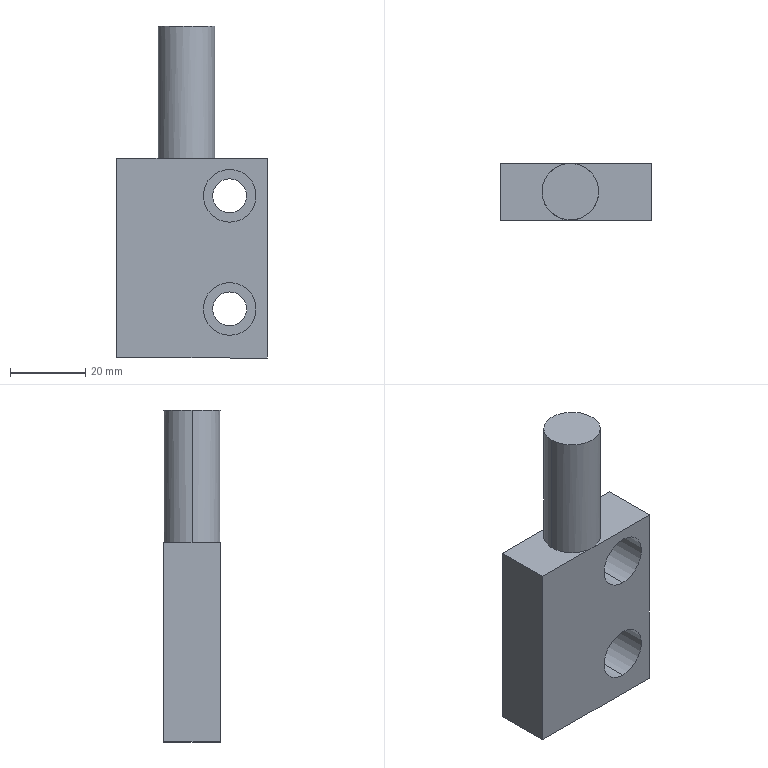Part | SolidWorks | features BaseBody 1 | 1 solid | 20 faces | box 40 x 15 x 88 mm | volume 34270 mm3 | cylinder 10 | plane 10 | commonest cylinder face diameters 9 x4 14 x4 15 x2
STEP:
#1=CARTESIAN_POINT('',(-340.,-80.,212.621));
#2=VERTEX_POINT('',#1);
#3=CARTESIAN_POINT('',(-340.,-80.,221.621));
#4=VERTEX_POINT('',#3);
#5=CARTESIAN_POINT('',(-340.,-80.,217.121));
#6=DIRECTION('',(0.,1.,0.));
#7=DIRECTION('',(0.,0.,-1.));
#8=AXIS2_PLACEMENT_3D('',#5,#6,#7);
#9=CIRCLE('',#8,4.5);
#10=EDGE_CURVE('',#2,#4,#9,.T.);
#11=ORIENTED_EDGE('',*,*,#10,.T.);
#12=CARTESIAN_POINT('',(-340.,-85.,221.621));
#13=VERTEX_POINT('',#12);
#14=CARTESIAN_POINT('',(-340.,-95.,221.621));
#15=DIRECTION('',(0.,-1.,0.));
#16=VECTOR('',#15,1000.);
#17=LINE('',#14,#16);
#18=EDGE_CURVE('',#4,#13,#17,.T.);
#19=ORIENTED_EDGE('',*,*,#18,.T.);
#20=CARTESIAN_POINT('',(-340.,-85.,212.621));
#21=VERTEX_POINT('',#20);
#22=CARTESIAN_POINT('',(-340.,-85.,217.121));
#23=DIRECTION('',(0.,1.,0.));
#24=DIRECTION('',(0.,0.,-1.));
#25=AXIS2_PLACEMENT_3D('',#22,#23,#24);
#26=CIRCLE('',#25,4.5);
#27=EDGE_CURVE('',#21,#13,#26,.T.);
#28=ORIENTED_EDGE('',*,*,#27,.F.);
#29=CARTESIAN_POINT('',(-340.,-95.,212.621));
#30=DIRECTION('',(0.,-1.,0.));
#31=VECTOR('',#30,1000.);
#32=LINE('',#29,#31);
#33=EDGE_CURVE('',#2,#21,#32,.T.);
#34=ORIENTED_EDGE('',*,*,#33,.F.);
#35=EDGE_LOOP('',(#11,#19,#28,#34));
#36=FACE_OUTER_BOUND('',#35,.T.);
#37=CARTESIAN_POINT('',(-340.,-95.,217.121));
#38=DIRECTION('',(0.,-1.,0.));
#39=DIRECTION('',(0.,0.,-1.));
#40=AXIS2_PLACEMENT_3D('',#37,#38,#39);
#41=CYLINDRICAL_SURFACE('',#40,4.5);
#42=ADVANCED_FACE('',(#36),#41,.F.);
#43=CARTESIAN_POINT('',(-340.,-80.,242.621));
#44=VERTEX_POINT('',#43);
#45=CARTESIAN_POINT('',(-340.,-80.,251.621));
#46=VERTEX_POINT('',#45);
#47=CARTESIAN_POINT('',(-340.,-80.,247.121));
#48=DIRECTION('',(0.,1.,0.));
#49=DIRECTION('',(0.,0.,-1.));
#50=AXIS2_PLACEMENT_3D('',#47,#48,#49);
#51=CIRCLE('',#50,4.5);
#52=EDGE_CURVE('',#44,#46,#51,.T.);
#53=ORIENTED_EDGE('',*,*,#52,.T.);
#54=CARTESIAN_POINT('',(-340.,-85.,251.621));
#55=VERTEX_POINT('',#54);
#56=CARTESIAN_POINT('',(-340.,-95.,251.621));
#57=DIRECTION('',(0.,-1.,0.));
#58=VECTOR('',#57,1000.);
#59=LINE('',#56,#58);
#60=EDGE_CURVE('',#46,#55,#59,.T.);
#61=ORIENTED_EDGE('',*,*,#60,.T.);
#62=CARTESIAN_POINT('',(-340.,-85.,242.621));
#63=VERTEX_POINT('',#62);
#64=CARTESIAN_POINT('',(-340.,-85.,247.121));
#65=DIRECTION('',(0.,1.,0.));
#66=DIRECTION('',(0.,0.,-1.));
#67=AXIS2_PLACEMENT_3D('',#64,#65,#66);
#68=CIRCLE('',#67,4.5);
#69=EDGE_CURVE('',#63,#55,#68,.T.);
#70=ORIENTED_EDGE('',*,*,#69,.F.);
#71=CARTESIAN_POINT('',(-340.,-95.,242.621));
#72=DIRECTION('',(0.,-1.,0.));
#73=VECTOR('',#72,1000.);
#74=LINE('',#71,#73);
#75=EDGE_CURVE('',#44,#63,#74,.T.);
#76=ORIENTED_EDGE('',*,*,#75,.F.);
#77=EDGE_LOOP('',(#53,#61,#70,#76));
#78=FACE_OUTER_BOUND('',#77,.T.);
#79=CARTESIAN_POINT('',(-340.,-95.,247.121));
#80=DIRECTION('',(0.,-1.,0.));
#81=DIRECTION('',(0.,0.,-1.));
#82=AXIS2_PLACEMENT_3D('',#79,#80,#81);
#83=CYLINDRICAL_SURFACE('',#82,4.5);
#84=ADVANCED_FACE('',(#78),#83,.F.);
#85=CARTESIAN_POINT('',(-359.,-87.5,292.121));
#86=VERTEX_POINT('',#85);
#87=CARTESIAN_POINT('',(-344.,-87.5,292.121));
#88=VERTEX_POINT('',#87);
#89=CARTESIAN_POINT('',(-351.5,-87.5,292.121));
#90=DIRECTION('',(0.,0.,-1.));
#91=DIRECTION('',(-1.,0.,0.));
#92=AXIS2_PLACEMENT_3D('',#89,#90,#91);
#93=CIRCLE('',#92,7.5);
#94=EDGE_CURVE('',#86,#88,#93,.T.);
#95=ORIENTED_EDGE('',*,*,#94,.T.);
#96=CARTESIAN_POINT('',(-344.,-87.5,257.121));
#97=VERTEX_POINT('',#96);
#98=CARTESIAN_POINT('',(-344.,-87.5,292.121));
#99=DIRECTION('',(0.,0.,-1.));
#100=VECTOR('',#99,1000.);
#101=LINE('',#98,#100);
#102=EDGE_CURVE('',#88,#97,#101,.T.);
#103=ORIENTED_EDGE('',*,*,#102,.T.);
#104=CARTESIAN_POINT('',(-351.5,-80.,257.121));
#105=VERTEX_POINT('',#104);
#106=CARTESIAN_POINT('',(-351.5,-87.5,257.121));
#107=DIRECTION('',(0.,0.,1.));
#108=DIRECTION('',(-1.,0.,0.));
#109=AXIS2_PLACEMENT_3D('',#106,#107,#108);
#110=CIRCLE('',#109,7.5);
#111=EDGE_CURVE('',#97,#105,#110,.T.);
#112=ORIENTED_EDGE('',*,*,#111,.T.);
#113=CARTESIAN_POINT('',(-359.,-87.5,257.121));
#114=VERTEX_POINT('',#113);
#115=CARTESIAN_POINT('',(-351.5,-87.5,257.121));
#116=DIRECTION('',(0.,0.,1.));
#117=DIRECTION('',(-1.,0.,0.));
#118=AXIS2_PLACEMENT_3D('',#115,#116,#117);
#119=CIRCLE('',#118,7.5);
#120=EDGE_CURVE('',#105,#114,#119,.T.);
#121=ORIENTED_EDGE('',*,*,#120,.T.);
#122=CARTESIAN_POINT('',(-359.,-87.5,292.121));
#123=DIRECTION('',(0.,0.,-1.));
#124=VECTOR('',#123,1000.);
#125=LINE('',#122,#124);
#126=EDGE_CURVE('',#86,#114,#125,.T.);
#127=ORIENTED_EDGE('',*,*,#126,.F.);
#128=EDGE_LOOP('',(#95,#103,#112,#121,#127));
#129=FACE_OUTER_BOUND('',#128,.T.);
#130=CARTESIAN_POINT('',(-351.5,-87.5,292.121));
#131=DIRECTION('',(0.,0.,-1.));
#132=DIRECTION('',(-1.,0.,0.));
#133=AXIS2_PLACEMENT_3D('',#130,#131,#132);
#134=CYLINDRICAL_SURFACE('',#133,7.5);
#135=ADVANCED_FACE('',(#129),#134,.T.);
#136=CARTESIAN_POINT('',(-340.,-85.,224.121));
#137=VERTEX_POINT('',#136);
#138=CARTESIAN_POINT('',(-340.,-85.,210.121));
#139=VERTEX_POINT('',#138);
#140=CARTESIAN_POINT('',(-340.,-85.,217.121));
#141=DIRECTION('',(0.,-1.,0.));
#142=DIRECTION('',(0.,0.,-1.));
#143=AXIS2_PLACEMENT_3D('',#140,#141,#142);
#144=CIRCLE('',#143,7.);
#145=EDGE_CURVE('',#137,#139,#144,.T.);
#146=ORIENTED_EDGE('',*,*,#145,.F.);
#147=CARTESIAN_POINT('',(-340.,-95.,224.121));
#148=VERTEX_POINT('',#147);
#149=CARTESIAN_POINT('',(-340.,-85.,224.121));
#150=DIRECTION('',(0.,-1.,0.));
#151=VECTOR('',#150,1000.);
#152=LINE('',#149,#151);
#153=EDGE_CURVE('',#137,#148,#152,.T.);
#154=ORIENTED_EDGE('',*,*,#153,.T.);
#155=CARTESIAN_POINT('',(-340.,-95.,210.121));
#156=VERTEX_POINT('',#155);
#157=CARTESIAN_POINT('',(-340.,-95.,217.121));
#158=DIRECTION('',(0.,-1.,0.));
#159=DIRECTION('',(0.,0.,-1.));
#160=AXIS2_PLACEMENT_3D('',#157,#158,#159);
#161=CIRCLE('',#160,7.);
#162=EDGE_CURVE('',#148,#156,#161,.T.);
#163=ORIENTED_EDGE('',*,*,#162,.T.);
#164=CARTESIAN_POINT('',(-340.,-85.,210.121));
#165=DIRECTION('',(0.,-1.,0.));
#166=VECTOR('',#165,1000.);
#167=LINE('',#164,#166);
#168=EDGE_CURVE('',#139,#156,#167,.T.);
#169=ORIENTED_EDGE('',*,*,#168,.F.);
#170=EDGE_LOOP('',(#146,#154,#163,#169));
#171=FACE_OUTER_BOUND('',#170,.T.);
#172=CARTESIAN_POINT('',(-340.,-85.,217.121));
#173=DIRECTION('',(0.,-1.,0.));
#174=DIRECTION('',(0.,0.,-1.));
#175=AXIS2_PLACEMENT_3D('',#172,#173,#174);
#176=CYLINDRICAL_SURFACE('',#175,7.);
#177=ADVANCED_FACE('',(#171),#176,.F.);
#178=CARTESIAN_POINT('',(-340.,-85.,254.121));
#179=VERTEX_POINT('',#178);
#180=CARTESIAN_POINT('',(-340.,-85.,240.121));
#181=VERTEX_POINT('',#180);
#182=CARTESIAN_POINT('',(-340.,-85.,247.121));
#183=DIRECTION('',(0.,-1.,0.));
#184=DIRECTION('',(0.,0.,-1.));
#185=AXIS2_PLACEMENT_3D('',#182,#183,#184);
#186=CIRCLE('',#185,7.);
#187=EDGE_CURVE('',#179,#181,#186,.T.);
#188=ORIENTED_EDGE('',*,*,#187,.F.);
#189=CARTESIAN_POINT('',(-340.,-95.,254.121));
#190=VERTEX_POINT('',#189);
#191=CARTESIAN_POINT('',(-340.,-85.,254.121));
#192=DIRECTION('',(0.,-1.,0.));
#193=VECTOR('',#192,1000.);
#194=LINE('',#191,#193);
#195=EDGE_CURVE('',#179,#190,#194,.T.);
#196=ORIENTED_EDGE('',*,*,#195,.T.);
#197=CARTESIAN_POINT('',(-340.,-95.,240.121));
#198=VERTEX_POINT('',#197);
#199=CARTESIAN_POINT('',(-340.,-95.,247.121));
#200=DIRECTION('',(0.,-1.,0.));
#201=DIRECTION('',(0.,0.,-1.));
#202=AXIS2_PLACEMENT_3D('',#199,#200,#201);
#203=CIRCLE('',#202,7.);
#204=EDGE_CURVE('',#190,#198,#203,.T.);
#205=ORIENTED_EDGE('',*,*,#204,.T.);
#206=CARTESIAN_POINT('',(-340.,-85.,240.121));
#207=DIRECTION('',(0.,-1.,0.));
#208=VECTOR('',#207,1000.);
#209=LINE('',#206,#208);
#210=EDGE_CURVE('',#181,#198,#209,.T.);
#211=ORIENTED_EDGE('',*,*,#210,.F.);
#212=EDGE_LOOP('',(#188,#196,#205,#211));
#213=FACE_OUTER_BOUND('',#212,.T.);
#214=CARTESIAN_POINT('',(-340.,-85.,247.121));
#215=DIRECTION('',(0.,-1.,0.));
#216=DIRECTION('',(0.,0.,-1.));
#217=AXIS2_PLACEMENT_3D('',#214,#215,#216);
#218=CYLINDRICAL_SURFACE('',#217,7.);
#219=ADVANCED_FACE('',(#213),#218,.F.);
#220=CARTESIAN_POINT('',(-370.,-80.,257.121));
#221=VERTEX_POINT('',#220);
#222=CARTESIAN_POINT('',(-370.,-80.,204.121));
#223=VERTEX_POINT('',#222);
#224=CARTESIAN_POINT('',(-370.,-80.,204.121));
#225=DIRECTION('',(0.,0.,-1.));
#226=VECTOR('',#225,1000.);
#227=LINE('',#224,#226);
#228=EDGE_CURVE('',#221,#223,#227,.T.);
#229=ORIENTED_EDGE('',*,*,#228,.F.);
#230=CARTESIAN_POINT('',(-330.,-80.,257.121));
#231=DIRECTION('',(-1.,0.,0.));
#232=VECTOR('',#231,1000.);
#233=LINE('',#230,#232);
#234=EDGE_CURVE('',#105,#221,#233,.T.);
#235=ORIENTED_EDGE('',*,*,#234,.F.);
#236=CARTESIAN_POINT('',(-330.,-80.,257.121));
#237=VERTEX_POINT('',#236);
#238=CARTESIAN_POINT('',(-330.,-80.,257.121));
#239=DIRECTION('',(-1.,0.,0.));
#240=VECTOR('',#239,1000.);
#241=LINE('',#238,#240);
#242=EDGE_CURVE('',#237,#105,#241,.T.);
#243=ORIENTED_EDGE('',*,*,#242,.F.);
#244=CARTESIAN_POINT('',(-330.,-80.,204.121));
#245=VERTEX_POINT('',#244);
#246=CARTESIAN_POINT('',(-330.,-80.,204.121));
#247=DIRECTION('',(0.,0.,1.));
#248=VECTOR('',#247,1000.);
#249=LINE('',#246,#248);
#250=EDGE_CURVE('',#245,#237,#249,.T.);
#251=ORIENTED_EDGE('',*,*,#250,.F.);
#252=CARTESIAN_POINT('',(-330.,-80.,204.121));
#253=DIRECTION('',(1.,0.,0.));
#254=VECTOR('',#253,1000.);
#255=LINE('',#252,#254);
#256=EDGE_CURVE('',#223,#245,#255,.T.);
#257=ORIENTED_EDGE('',*,*,#256,.F.);
#258=EDGE_LOOP('',(#229,#235,#243,#251,#257));
#259=FACE_OUTER_BOUND('',#258,.T.);
#260=ORIENTED_EDGE('',*,*,#10,.F.);
#261=CARTESIAN_POINT('',(-340.,-80.,217.121));
#262=DIRECTION('',(0.,1.,0.));
#263=DIRECTION('',(0.,0.,-1.));
#264=AXIS2_PLACEMENT_3D('',#261,#262,#263);
#265=CIRCLE('',#264,4.5);
#266=EDGE_CURVE('',#4,#2,#265,.T.);
#267=ORIENTED_EDGE('',*,*,#266,.F.);
#268=EDGE_LOOP('',(#260,#267));
#269=FACE_BOUND('',#268,.T.);
#270=ORIENTED_EDGE('',*,*,#52,.F.);
#271=CARTESIAN_POINT('',(-340.,-80.,247.121));
#272=DIRECTION('',(0.,1.,0.));
#273=DIRECTION('',(0.,0.,-1.));
#274=AXIS2_PLACEMENT_3D('',#271,#272,#273);
#275=CIRCLE('',#274,4.5);
#276=EDGE_CURVE('',#46,#44,#275,.T.);
#277=ORIENTED_EDGE('',*,*,#276,.F.);
#278=EDGE_LOOP('',(#270,#277));
#279=FACE_BOUND('',#278,.T.);
#280=CARTESIAN_POINT('',(-330.,-80.,204.121));
#281=DIRECTION('',(0.,-1.,0.));
#282=DIRECTION('',(0.,0.,-1.));
#283=AXIS2_PLACEMENT_3D('',#280,#281,#282);
#284=PLANE('',#283);
#285=ADVANCED_FACE('',(#259,#269,#279),#284,.F.);
#286=CARTESIAN_POINT('',(-370.,-95.,204.121));
#287=VERTEX_POINT('',#286);
#288=CARTESIAN_POINT('',(-370.,-95.,204.121));
#289=DIRECTION('',(0.,-1.,0.));
#290=VECTOR('',#289,1000.);
#291=LINE('',#288,#290);
#292=EDGE_CURVE('',#223,#287,#291,.T.);
#293=ORIENTED_EDGE('',*,*,#292,.F.);
#294=ORIENTED_EDGE('',*,*,#256,.T.);
#295=CARTESIAN_POINT('',(-330.,-95.,204.121));
#296=VERTEX_POINT('',#295);
#297=CARTESIAN_POINT('',(-330.,-95.,204.121));
#298=DIRECTION('',(0.,1.,0.));
#299=VECTOR('',#298,1000.);
#300=LINE('',#297,#299);
#301=EDGE_CURVE('',#296,#245,#300,.T.);
#302=ORIENTED_EDGE('',*,*,#301,.F.);
#303=CARTESIAN_POINT('',(-330.,-95.,204.121));
#304=DIRECTION('',(1.,0.,0.));
#305=VECTOR('',#304,1000.);
#306=LINE('',#303,#305);
#307=EDGE_CURVE('',#287,#296,#306,.T.);
#308=ORIENTED_EDGE('',*,*,#307,.F.);
#309=EDGE_LOOP('',(#293,#294,#302,#308));
#310=FACE_OUTER_BOUND('',#309,.T.);
#311=CARTESIAN_POINT('',(-330.,-95.,204.121));
#312=DIRECTION('',(0.,0.,1.));
#313=DIRECTION('',(1.,0.,0.));
#314=AXIS2_PLACEMENT_3D('',#311,#312,#313);
#315=PLANE('',#314);
#316=ADVANCED_FACE('',(#310),#315,.F.);
#317=ORIENTED_EDGE('',*,*,#228,.T.);
#318=ORIENTED_EDGE('',*,*,#292,.T.);
#319=CARTESIAN_POINT('',(-370.,-95.,257.121));
#320=VERTEX_POINT('',#319);
#321=CARTESIAN_POINT('',(-370.,-95.,230.621));
#322=DIRECTION('',(0.,0.,1.));
#323=VECTOR('',#322,1000.);
#324=LINE('',#321,#323);
#325=EDGE_CURVE('',#287,#320,#324,.T.);
#326=ORIENTED_EDGE('',*,*,#325,.T.);
#327=CARTESIAN_POINT('',(-370.,-87.5,257.121));
#328=DIRECTION('',(0.,1.,0.));
#329=VECTOR('',#328,1000.);
#330=LINE('',#327,#329);
#331=EDGE_CURVE('',#320,#221,#330,.T.);
#332=ORIENTED_EDGE('',*,*,#331,.T.);
#333=EDGE_LOOP('',(#317,#318,#326,#332));
#334=FACE_OUTER_BOUND('',#333,.T.);
#335=CARTESIAN_POINT('',(-370.,-87.5,230.621));
#336=DIRECTION('',(-1.,0.,0.));
#337=DIRECTION('',(0.,0.,1.));
#338=AXIS2_PLACEMENT_3D('',#335,#336,#337);
#339=PLANE('',#338);
#340=ADVANCED_FACE('',(#334),#339,.T.);
#341=ORIENTED_EDGE('',*,*,#120,.F.);
#342=ORIENTED_EDGE('',*,*,#234,.T.);
#343=ORIENTED_EDGE('',*,*,#331,.F.);
#344=CARTESIAN_POINT('',(-351.5,-95.,257.121));
#345=VERTEX_POINT('',#344);
#346=CARTESIAN_POINT('',(-330.,-95.,257.121));
#347=DIRECTION('',(-1.,0.,0.));
#348=VECTOR('',#347,1000.);
#349=LINE('',#346,#348);
#350=EDGE_CURVE('',#345,#320,#349,.T.);
#351=ORIENTED_EDGE('',*,*,#350,.F.);
#352=CARTESIAN_POINT('',(-351.5,-87.5,257.121));
#353=DIRECTION('',(0.,0.,1.));
#354=DIRECTION('',(-1.,0.,0.));
#355=AXIS2_PLACEMENT_3D('',#352,#353,#354);
#356=CIRCLE('',#355,7.5);
#357=EDGE_CURVE('',#114,#345,#356,.T.);
#358=ORIENTED_EDGE('',*,*,#357,.F.);
#359=EDGE_LOOP('',(#341,#342,#343,#351,#358));
#360=FACE_OUTER_BOUND('',#359,.T.);
#361=CARTESIAN_POINT('',(-330.,-95.,257.121));
#362=DIRECTION('',(0.,0.,-1.));
#363=DIRECTION('',(-1.,0.,0.));
#364=AXIS2_PLACEMENT_3D('',#361,#362,#363);
#365=PLANE('',#364);
#366=ADVANCED_FACE('',(#360),#365,.F.);
#367=CARTESIAN_POINT('',(-351.5,-87.5,257.121));
#368=DIRECTION('',(0.,0.,1.));
#369=DIRECTION('',(-1.,0.,0.));
#370=AXIS2_PLACEMENT_3D('',#367,#368,#369);
#371=CIRCLE('',#370,7.5);
#372=EDGE_CURVE('',#345,#97,#371,.T.);
#373=ORIENTED_EDGE('',*,*,#372,.F.);
#374=CARTESIAN_POINT('',(-330.,-95.,257.121));
#375=VERTEX_POINT('',#374);
#376=CARTESIAN_POINT('',(-330.,-95.,257.121));
#377=DIRECTION('',(-1.,0.,0.));
#378=VECTOR('',#377,1000.);
#379=LINE('',#376,#378);
#380=EDGE_CURVE('',#375,#345,#379,.T.);
#381=ORIENTED_EDGE('',*,*,#380,.F.);
#382=CARTESIAN_POINT('',(-330.,-95.,257.121));
#383=DIRECTION('',(0.,-1.,0.));
#384=VECTOR('',#383,1000.);
#385=LINE('',#382,#384);
#386=EDGE_CURVE('',#237,#375,#385,.T.);
#387=ORIENTED_EDGE('',*,*,#386,.F.);
#388=ORIENTED_EDGE('',*,*,#242,.T.);
#389=ORIENTED_EDGE('',*,*,#111,.F.);
#390=EDGE_LOOP('',(#373,#381,#387,#388,#389));
#391=FACE_OUTER_BOUND('',#390,.T.);
#392=CARTESIAN_POINT('',(-330.,-95.,257.121));
#393=DIRECTION('',(0.,0.,-1.));
#394=DIRECTION('',(-1.,0.,0.));
#395=AXIS2_PLACEMENT_3D('',#392,#393,#394);
#396=PLANE('',#395);
#397=ADVANCED_FACE('',(#391),#396,.F.);
#398=ORIENTED_EDGE('',*,*,#301,.T.);
#399=ORIENTED_EDGE('',*,*,#250,.T.);
#400=ORIENTED_EDGE('',*,*,#386,.T.);
#401=CARTESIAN_POINT('',(-330.,-95.,230.621));
#402=DIRECTION('',(0.,0.,-1.));
#403=VECTOR('',#402,1000.);
#404=LINE('',#401,#403);
#405=EDGE_CURVE('',#375,#296,#404,.T.);
#406=ORIENTED_EDGE('',*,*,#405,.T.);
#407=EDGE_LOOP('',(#398,#399,#400,#406));
#408=FACE_OUTER_BOUND('',#407,.T.);
#409=CARTESIAN_POINT('',(-330.,-87.5,230.621));
#410=DIRECTION('',(1.,0.,0.));
#411=DIRECTION('',(0.,0.,-1.));
#412=AXIS2_PLACEMENT_3D('',#409,#410,#411);
#413=PLANE('',#412);
#414=ADVANCED_FACE('',(#408),#413,.T.);
#415=ORIENTED_EDGE('',*,*,#18,.F.);
#416=ORIENTED_EDGE('',*,*,#266,.T.);
#417=ORIENTED_EDGE('',*,*,#33,.T.);
#418=CARTESIAN_POINT('',(-340.,-85.,217.121));
#419=DIRECTION('',(0.,1.,0.));
#420=DIRECTION('',(0.,0.,-1.));
#421=AXIS2_PLACEMENT_3D('',#418,#419,#420);
#422=CIRCLE('',#421,4.5);
#423=EDGE_CURVE('',#13,#21,#422,.T.);
#424=ORIENTED_EDGE('',*,*,#423,.F.);
#425=EDGE_LOOP('',(#415,#416,#417,#424));
#426=FACE_OUTER_BOUND('',#425,.T.);
#427=CARTESIAN_POINT('',(-340.,-95.,217.121));
#428=DIRECTION('',(0.,-1.,0.));
#429=DIRECTION('',(0.,0.,-1.));
#430=AXIS2_PLACEMENT_3D('',#427,#428,#429);
#431=CYLINDRICAL_SURFACE('',#430,4.5);
#432=ADVANCED_FACE('',(#426),#431,.F.);
#433=ORIENTED_EDGE('',*,*,#60,.F.);
#434=ORIENTED_EDGE('',*,*,#276,.T.);
#435=ORIENTED_EDGE('',*,*,#75,.T.);
#436=CARTESIAN_POINT('',(-340.,-85.,247.121));
#437=DIRECTION('',(0.,1.,0.));
#438=DIRECTION('',(0.,0.,-1.));
#439=AXIS2_PLACEMENT_3D('',#436,#437,#438);
#440=CIRCLE('',#439,4.5);
#441=EDGE_CURVE('',#55,#63,#440,.T.);
#442=ORIENTED_EDGE('',*,*,#441,.F.);
#443=EDGE_LOOP('',(#433,#434,#435,#442));
#444=FACE_OUTER_BOUND('',#443,.T.);
#445=CARTESIAN_POINT('',(-340.,-95.,247.121));
#446=DIRECTION('',(0.,-1.,0.));
#447=DIRECTION('',(0.,0.,-1.));
#448=AXIS2_PLACEMENT_3D('',#445,#446,#447);
#449=CYLINDRICAL_SURFACE('',#448,4.5);
#450=ADVANCED_FACE('',(#444),#449,.F.);
#451=ORIENTED_EDGE('',*,*,#350,.T.);
#452=ORIENTED_EDGE('',*,*,#325,.F.);
#453=ORIENTED_EDGE('',*,*,#307,.T.);
#454=ORIENTED_EDGE('',*,*,#405,.F.);
#455=ORIENTED_EDGE('',*,*,#380,.T.);
#456=EDGE_LOOP('',(#451,#452,#453,#454,#455));
#457=FACE_OUTER_BOUND('',#456,.T.);
#458=CARTESIAN_POINT('',(-340.,-95.,217.121));
#459=DIRECTION('',(0.,-1.,0.));
#460=DIRECTION('',(0.,0.,-1.));
#461=AXIS2_PLACEMENT_3D('',#458,#459,#460);
#462=CIRCLE('',#461,7.);
#463=EDGE_CURVE('',#156,#148,#462,.T.);
#464=ORIENTED_EDGE('',*,*,#463,.F.);
#465=ORIENTED_EDGE('',*,*,#162,.F.);
#466=EDGE_LOOP('',(#464,#465));
#467=FACE_BOUND('',#466,.T.);
#468=CARTESIAN_POINT('',(-340.,-95.,247.121));
#469=DIRECTION('',(0.,-1.,0.));
#470=DIRECTION('',(0.,0.,-1.));
#471=AXIS2_PLACEMENT_3D('',#468,#469,#470);
#472=CIRCLE('',#471,7.);
#473=EDGE_CURVE('',#198,#190,#472,.T.);
#474=ORIENTED_EDGE('',*,*,#473,.F.);
#475=ORIENTED_EDGE('',*,*,#204,.F.);
#476=EDGE_LOOP('',(#474,#475));
#477=FACE_BOUND('',#476,.T.);
#478=CARTESIAN_POINT('',(-330.,-95.,204.121));
#479=DIRECTION('',(0.,1.,0.));
#480=DIRECTION('',(0.,0.,1.));
#481=AXIS2_PLACEMENT_3D('',#478,#479,#480);
#482=PLANE('',#481);
#483=ADVANCED_FACE('',(#457,#467,#477),#482,.F.);
#484=ORIENTED_EDGE('',*,*,#102,.F.);
#485=CARTESIAN_POINT('',(-351.5,-87.5,292.121));
#486=DIRECTION('',(0.,0.,-1.));
#487=DIRECTION('',(-1.,0.,0.));
#488=AXIS2_PLACEMENT_3D('',#485,#486,#487);
#489=CIRCLE('',#488,7.5);
#490=EDGE_CURVE('',#88,#86,#489,.T.);
#491=ORIENTED_EDGE('',*,*,#490,.T.);
#492=ORIENTED_EDGE('',*,*,#126,.T.);
#493=ORIENTED_EDGE('',*,*,#357,.T.);
#494=ORIENTED_EDGE('',*,*,#372,.T.);
#495=EDGE_LOOP('',(#484,#491,#492,#493,#494));
#496=FACE_OUTER_BOUND('',#495,.T.);
#497=CARTESIAN_POINT('',(-351.5,-87.5,292.121));
#498=DIRECTION('',(0.,0.,-1.));
#499=DIRECTION('',(-1.,0.,0.));
#500=AXIS2_PLACEMENT_3D('',#497,#498,#499);
#501=CYLINDRICAL_SURFACE('',#500,7.5);
#502=ADVANCED_FACE('',(#496),#501,.T.);
#503=ORIENTED_EDGE('',*,*,#27,.T.);
#504=ORIENTED_EDGE('',*,*,#423,.T.);
#505=EDGE_LOOP('',(#503,#504));
#506=FACE_BOUND('',#505,.T.);
#507=CARTESIAN_POINT('',(-340.,-85.,217.121));
#508=DIRECTION('',(0.,-1.,0.));
#509=DIRECTION('',(0.,0.,-1.));
#510=AXIS2_PLACEMENT_3D('',#507,#508,#509);
#511=CIRCLE('',#510,7.);
#512=EDGE_CURVE('',#139,#137,#511,.T.);
#513=ORIENTED_EDGE('',*,*,#512,.T.);
#514=ORIENTED_EDGE('',*,*,#145,.T.);
#515=EDGE_LOOP('',(#513,#514));
#516=FACE_OUTER_BOUND('',#515,.T.);
#517=CARTESIAN_POINT('',(-340.,-85.,217.121));
#518=DIRECTION('',(0.,-1.,0.));
#519=DIRECTION('',(0.,0.,-1.));
#520=AXIS2_PLACEMENT_3D('',#517,#518,#519);
#521=PLANE('',#520);
#522=ADVANCED_FACE('',(#506,#516),#521,.T.);
#523=ORIENTED_EDGE('',*,*,#69,.T.);
#524=ORIENTED_EDGE('',*,*,#441,.T.);
#525=EDGE_LOOP('',(#523,#524));
#526=FACE_BOUND('',#525,.T.);
#527=CARTESIAN_POINT('',(-340.,-85.,247.121));
#528=DIRECTION('',(0.,-1.,0.));
#529=DIRECTION('',(0.,0.,-1.));
#530=AXIS2_PLACEMENT_3D('',#527,#528,#529);
#531=CIRCLE('',#530,7.);
#532=EDGE_CURVE('',#181,#179,#531,.T.);
#533=ORIENTED_EDGE('',*,*,#532,.T.);
#534=ORIENTED_EDGE('',*,*,#187,.T.);
#535=EDGE_LOOP('',(#533,#534));
#536=FACE_OUTER_BOUND('',#535,.T.);
#537=CARTESIAN_POINT('',(-340.,-85.,247.121));
#538=DIRECTION('',(0.,-1.,0.));
#539=DIRECTION('',(0.,0.,-1.));
#540=AXIS2_PLACEMENT_3D('',#537,#538,#539);
#541=PLANE('',#540);
#542=ADVANCED_FACE('',(#526,#536),#541,.T.);
#543=ORIENTED_EDGE('',*,*,#153,.F.);
#544=ORIENTED_EDGE('',*,*,#512,.F.);
#545=ORIENTED_EDGE('',*,*,#168,.T.);
#546=ORIENTED_EDGE('',*,*,#463,.T.);
#547=EDGE_LOOP('',(#543,#544,#545,#546));
#548=FACE_OUTER_BOUND('',#547,.T.);
#549=CARTESIAN_POINT('',(-340.,-85.,217.121));
#550=DIRECTION('',(0.,-1.,0.));
#551=DIRECTION('',(0.,0.,-1.));
#552=AXIS2_PLACEMENT_3D('',#549,#550,#551);
#553=CYLINDRICAL_SURFACE('',#552,7.);
#554=ADVANCED_FACE('',(#548),#553,.F.);
#555=ORIENTED_EDGE('',*,*,#195,.F.);
#556=ORIENTED_EDGE('',*,*,#532,.F.);
#557=ORIENTED_EDGE('',*,*,#210,.T.);
#558=ORIENTED_EDGE('',*,*,#473,.T.);
#559=EDGE_LOOP('',(#555,#556,#557,#558));
#560=FACE_OUTER_BOUND('',#559,.T.);
#561=CARTESIAN_POINT('',(-340.,-85.,247.121));
#562=DIRECTION('',(0.,-1.,0.));
#563=DIRECTION('',(0.,0.,-1.));
#564=AXIS2_PLACEMENT_3D('',#561,#562,#563);
#565=CYLINDRICAL_SURFACE('',#564,7.);
#566=ADVANCED_FACE('',(#560),#565,.F.);
#567=ORIENTED_EDGE('',*,*,#94,.F.);
#568=ORIENTED_EDGE('',*,*,#490,.F.);
#569=EDGE_LOOP('',(#567,#568));
#570=FACE_OUTER_BOUND('',#569,.T.);
#571=CARTESIAN_POINT('',(-351.5,-87.5,292.121));
#572=DIRECTION('',(0.,0.,1.));
#573=DIRECTION('',(1.,0.,0.));
#574=AXIS2_PLACEMENT_3D('',#571,#572,#573);
#575=PLANE('',#574);
#576=ADVANCED_FACE('',(#570),#575,.T.);
#577=CLOSED_SHELL('',(#42,#84,#135,#177,#219,#285,#316,#340,#366,#397,#414,#432,#450,#483,#502,#522,#542,#554,#566,#576));
#578=MANIFOLD_SOLID_BREP('',#577);
#579=CARTESIAN_POINT('',(0.,0.,0.));
#580=DIRECTION('',(0.,0.,1.));
#581=DIRECTION('',(1.,0.,0.));
#582=AXIS2_PLACEMENT_3D('',#579,#580,#581);
#583=(LENGTH_UNIT()NAMED_UNIT(*)SI_UNIT(.MILLI.,.METRE.));
#584=UNCERTAINTY_MEASURE_WITH_UNIT(LENGTH_MEASURE(0.00001),#583,'','');
#585=(NAMED_UNIT(*)PLANE_ANGLE_UNIT()SI_UNIT($,.RADIAN.));
#586=(NAMED_UNIT(*)SI_UNIT($,.STERADIAN.)SOLID_ANGLE_UNIT());
#587=(GEOMETRIC_REPRESENTATION_CONTEXT(3)GLOBAL_UNCERTAINTY_ASSIGNED_CONTEXT((#584))GLOBAL_UNIT_ASSIGNED_CONTEXT((#583,#585,#586))REPRESENTATION_CONTEXT('',''));
#588=ADVANCED_BREP_SHAPE_REPRESENTATION('',(#578,#582),#587);